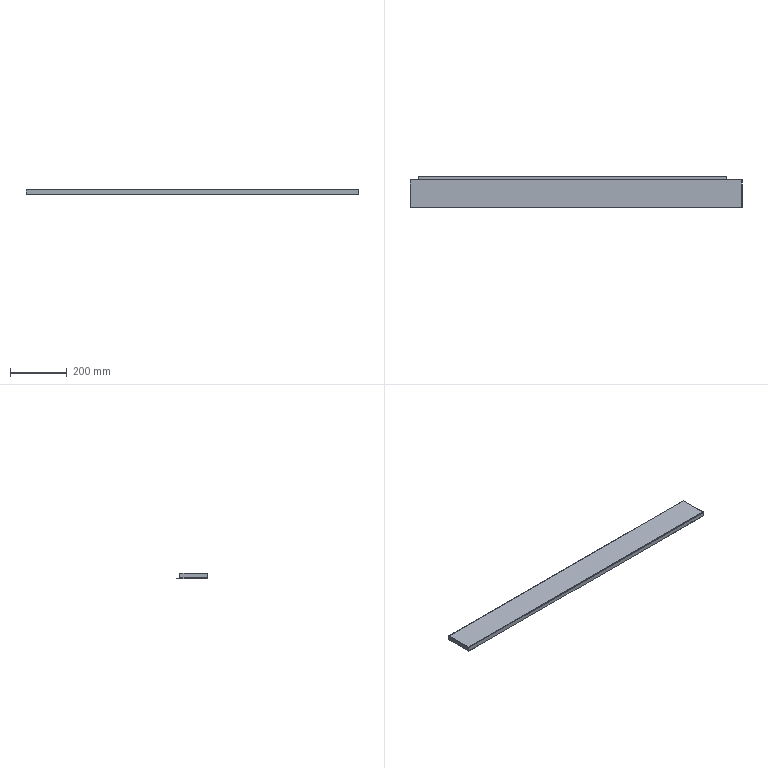Part | NX | features BREP 3 | 3 solids | 86 faces | box 1169 x 112 x 18 mm | volume 262597 mm3 | plane 72 | cylinder 14 | commonest cylinder face diameters 0.02 x7 3.02 x7